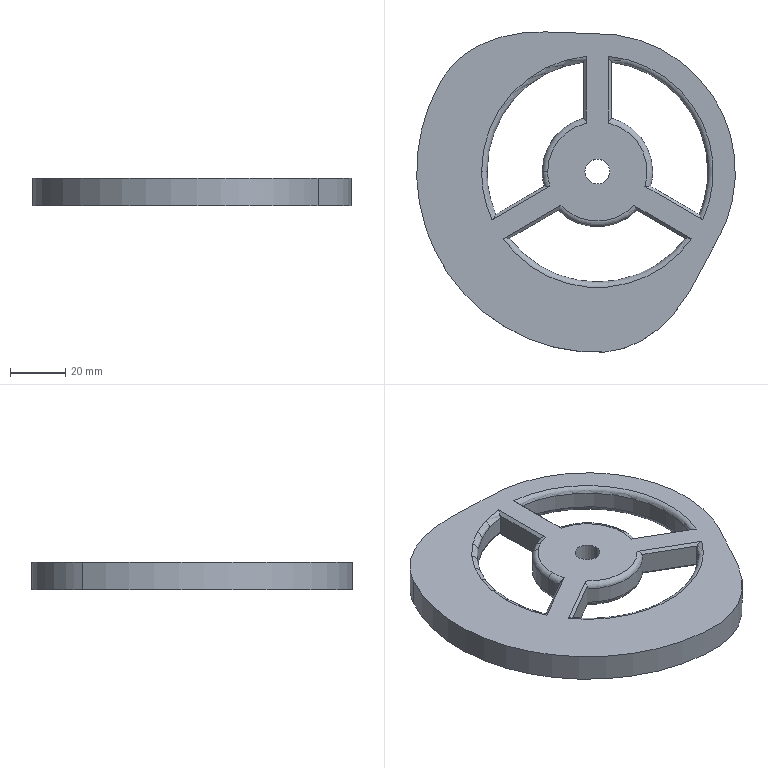Part | SolidWorks | features Fillet 2, Chamfer 1, Extrusion 1, ICE 1 | 1 solid | 48 faces | box 115.52 x 116.155 x 10 mm | volume 73313 mm3 | plane 20 | torus 16 | cylinder 10 | spline 2 | commonest cylinder face diameters 40 x4 80 x4 9 x2